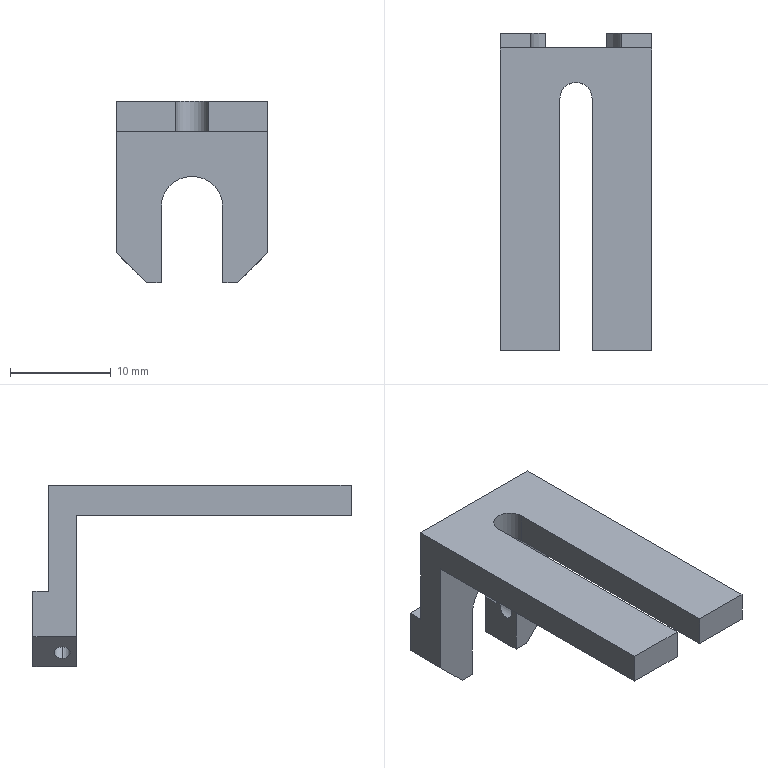Part | SolidWorks | features ICE 6, Extrusion 1, HoleWzd 1, MirrorPattern 1 | 1 solid | 28 faces | box 15 x 31.5 x 18 mm | volume 1594 mm3 | plane 20 | cylinder 8 | commonest cylinder face diameters 1.6 x4 9 x2 3.2 x1 6.1 x1
STEP:
#1=CARTESIAN_POINT('',(-3.05,1.4,-4.353));
#2=VERTEX_POINT('',#1);
#3=CARTESIAN_POINT('',(-3.05,1.4,-2.09));
#4=VERTEX_POINT('',#3);
#5=CARTESIAN_POINT('',(-3.05,1.4,-4.353));
#6=CARTESIAN_POINT('',(-3.05,-0.2,-4.353));
#7=CARTESIAN_POINT('',(-3.05,-0.2,-2.09));
#8=CARTESIAN_POINT('',(-3.05,1.4,-2.09));
#9=(BOUNDED_CURVE()B_SPLINE_CURVE(3,(#5,#6,#7,#8),.UNSPECIFIED.,.F.,.T.)B_SPLINE_CURVE_WITH_KNOTS((4,4),(0.,3.142),.UNSPECIFIED.)CURVE()GEOMETRIC_REPRESENTATION_ITEM()RATIONAL_B_SPLINE_CURVE((1.,0.3333,0.3333,1.))REPRESENTATION_ITEM(''));
#10=EDGE_CURVE('',#2,#4,#9,.T.);
#11=ORIENTED_EDGE('',*,*,#10,.F.);
#12=CARTESIAN_POINT('',(-5.349,1.4,-6.651));
#13=VERTEX_POINT('',#12);
#14=CARTESIAN_POINT('',(-5.349,1.4,-6.651));
#15=DIRECTION('',(-0.7071,0.,-0.7071));
#16=VECTOR('',#15,1000.);
#17=LINE('',#14,#16);
#18=EDGE_CURVE('',#2,#13,#17,.T.);
#19=ORIENTED_EDGE('',*,*,#18,.T.);
#20=CARTESIAN_POINT('',(-6.48,1.4,-5.52));
#21=VERTEX_POINT('',#20);
#22=CARTESIAN_POINT('',(-5.914,1.4,-6.086));
#23=DIRECTION('',(-0.7071,0.,-0.7071));
#24=DIRECTION('',(-0.7071,0.,0.7071));
#25=AXIS2_PLACEMENT_3D('',#22,#23,#24);
#26=CIRCLE('',#25,0.8);
#27=EDGE_CURVE('',#13,#21,#26,.T.);
#28=ORIENTED_EDGE('',*,*,#27,.T.);
#29=CARTESIAN_POINT('',(-6.48,1.4,-5.52));
#30=DIRECTION('',(-0.7071,0.,-0.7071));
#31=VECTOR('',#30,1000.);
#32=LINE('',#29,#31);
#33=EDGE_CURVE('',#4,#21,#32,.T.);
#34=ORIENTED_EDGE('',*,*,#33,.F.);
#35=EDGE_LOOP('',(#11,#19,#28,#34));
#36=FACE_OUTER_BOUND('',#35,.T.);
#37=CARTESIAN_POINT('',(-5.914,1.4,-6.086));
#38=DIRECTION('',(-0.7071,0.,-0.7071));
#39=DIRECTION('',(-0.7071,0.,0.7071));
#40=AXIS2_PLACEMENT_3D('',#37,#38,#39);
#41=CYLINDRICAL_SURFACE('',#40,0.8);
#42=ADVANCED_FACE('',(#36),#41,.F.);
#43=CARTESIAN_POINT('',(3.05,1.4,-2.09));
#44=VERTEX_POINT('',#43);
#45=CARTESIAN_POINT('',(3.05,1.4,-4.353));
#46=VERTEX_POINT('',#45);
#47=CARTESIAN_POINT('',(3.05,1.4,-2.09));
#48=CARTESIAN_POINT('',(3.05,-0.2,-2.09));
#49=CARTESIAN_POINT('',(3.05,-0.2,-4.353));
#50=CARTESIAN_POINT('',(3.05,1.4,-4.353));
#51=(BOUNDED_CURVE()B_SPLINE_CURVE(3,(#47,#48,#49,#50),.UNSPECIFIED.,.F.,.T.)B_SPLINE_CURVE_WITH_KNOTS((4,4),(3.142,6.283),.UNSPECIFIED.)CURVE()GEOMETRIC_REPRESENTATION_ITEM()RATIONAL_B_SPLINE_CURVE((1.,0.3333,0.3333,1.))REPRESENTATION_ITEM(''));
#52=EDGE_CURVE('',#44,#46,#51,.T.);
#53=ORIENTED_EDGE('',*,*,#52,.F.);
#54=CARTESIAN_POINT('',(6.48,1.4,-5.52));
#55=VERTEX_POINT('',#54);
#56=CARTESIAN_POINT('',(6.48,1.4,-5.52));
#57=DIRECTION('',(0.7071,0.,-0.7071));
#58=VECTOR('',#57,1000.);
#59=LINE('',#56,#58);
#60=EDGE_CURVE('',#44,#55,#59,.T.);
#61=ORIENTED_EDGE('',*,*,#60,.T.);
#62=CARTESIAN_POINT('',(5.349,1.4,-6.651));
#63=VERTEX_POINT('',#62);
#64=CARTESIAN_POINT('',(5.914,1.4,-6.086));
#65=DIRECTION('',(0.7071,0.,-0.7071));
#66=DIRECTION('',(-0.7071,0.,-0.7071));
#67=AXIS2_PLACEMENT_3D('',#64,#65,#66);
#68=CIRCLE('',#67,0.8);
#69=EDGE_CURVE('',#55,#63,#68,.T.);
#70=ORIENTED_EDGE('',*,*,#69,.T.);
#71=CARTESIAN_POINT('',(5.349,1.4,-6.651));
#72=DIRECTION('',(0.7071,0.,-0.7071));
#73=VECTOR('',#72,1000.);
#74=LINE('',#71,#73);
#75=EDGE_CURVE('',#46,#63,#74,.T.);
#76=ORIENTED_EDGE('',*,*,#75,.F.);
#77=EDGE_LOOP('',(#53,#61,#70,#76));
#78=FACE_OUTER_BOUND('',#77,.T.);
#79=CARTESIAN_POINT('',(5.914,1.4,-6.086));
#80=DIRECTION('',(0.7071,0.,-0.7071));
#81=DIRECTION('',(-0.7071,0.,-0.7071));
#82=AXIS2_PLACEMENT_3D('',#79,#80,#81);
#83=CYLINDRICAL_SURFACE('',#82,0.8);
#84=ADVANCED_FACE('',(#78),#83,.F.);
#85=CARTESIAN_POINT('',(1.6,-27.2,10.5));
#86=VERTEX_POINT('',#85);
#87=CARTESIAN_POINT('',(7.5,-27.2,10.5));
#88=VERTEX_POINT('',#87);
#89=CARTESIAN_POINT('',(-7.5,-27.2,10.5));
#90=DIRECTION('',(1.,0.,0.));
#91=VECTOR('',#90,1000.);
#92=LINE('',#89,#91);
#93=EDGE_CURVE('',#86,#88,#92,.T.);
#94=ORIENTED_EDGE('',*,*,#93,.F.);
#95=CARTESIAN_POINT('',(1.6,-27.2,7.5));
#96=VERTEX_POINT('',#95);
#97=CARTESIAN_POINT('',(1.6,-27.2,240.5));
#98=DIRECTION('',(0.,0.,-1.));
#99=VECTOR('',#98,1000.);
#100=LINE('',#97,#99);
#101=EDGE_CURVE('',#86,#96,#100,.T.);
#102=ORIENTED_EDGE('',*,*,#101,.T.);
#103=CARTESIAN_POINT('',(7.5,-27.2,7.5));
#104=VERTEX_POINT('',#103);
#105=CARTESIAN_POINT('',(-7.5,-27.2,7.5));
#106=DIRECTION('',(1.,0.,0.));
#107=VECTOR('',#106,1000.);
#108=LINE('',#105,#107);
#109=EDGE_CURVE('',#96,#104,#108,.T.);
#110=ORIENTED_EDGE('',*,*,#109,.T.);
#111=CARTESIAN_POINT('',(7.5,-27.2,10.5));
#112=DIRECTION('',(0.,0.,-1.));
#113=VECTOR('',#112,1000.);
#114=LINE('',#111,#113);
#115=EDGE_CURVE('',#88,#104,#114,.T.);
#116=ORIENTED_EDGE('',*,*,#115,.F.);
#117=EDGE_LOOP('',(#94,#102,#110,#116));
#118=FACE_OUTER_BOUND('',#117,.T.);
#119=CARTESIAN_POINT('',(-7.5,-27.2,10.5));
#120=DIRECTION('',(0.,1.,0.));
#121=DIRECTION('',(0.,0.,1.));
#122=AXIS2_PLACEMENT_3D('',#119,#120,#121);
#123=PLANE('',#122);
#124=ADVANCED_FACE('',(#118),#123,.F.);
#125=CARTESIAN_POINT('',(4.5,2.8,0.));
#126=VERTEX_POINT('',#125);
#127=CARTESIAN_POINT('',(7.5,2.8,0.));
#128=VERTEX_POINT('',#127);
#129=CARTESIAN_POINT('',(0.,2.8,0.));
#130=DIRECTION('',(1.,0.,0.));
#131=VECTOR('',#130,1000.);
#132=LINE('',#129,#131);
#133=EDGE_CURVE('',#126,#128,#132,.T.);
#134=ORIENTED_EDGE('',*,*,#133,.F.);
#135=CARTESIAN_POINT('',(3.05,2.8,-3.309));
#136=VERTEX_POINT('',#135);
#137=CARTESIAN_POINT('',(0.,2.8,0.));
#138=DIRECTION('',(0.,1.,0.));
#139=DIRECTION('',(0.,0.,1.));
#140=AXIS2_PLACEMENT_3D('',#137,#138,#139);
#141=CIRCLE('',#140,4.5);
#142=EDGE_CURVE('',#126,#136,#141,.T.);
#143=ORIENTED_EDGE('',*,*,#142,.T.);
#144=CARTESIAN_POINT('',(3.05,2.8,0.));
#145=VERTEX_POINT('',#144);
#146=CARTESIAN_POINT('',(3.05,2.8,-7.5));
#147=DIRECTION('',(0.,0.,1.));
#148=VECTOR('',#147,1000.);
#149=LINE('',#146,#148);
#150=EDGE_CURVE('',#136,#145,#149,.T.);
#151=ORIENTED_EDGE('',*,*,#150,.T.);
#152=CARTESIAN_POINT('',(-3.05,2.8,0.));
#153=VERTEX_POINT('',#152);
#154=CARTESIAN_POINT('',(0.,2.8,0.));
#155=DIRECTION('',(0.,-1.,0.));
#156=DIRECTION('',(0.,0.,1.));
#157=AXIS2_PLACEMENT_3D('',#154,#155,#156);
#158=CIRCLE('',#157,3.05);
#159=EDGE_CURVE('',#145,#153,#158,.T.);
#160=ORIENTED_EDGE('',*,*,#159,.T.);
#161=CARTESIAN_POINT('',(-3.05,2.8,-3.309));
#162=VERTEX_POINT('',#161);
#163=CARTESIAN_POINT('',(-3.05,2.8,0.));
#164=DIRECTION('',(0.,0.,-1.));
#165=VECTOR('',#164,1000.);
#166=LINE('',#163,#165);
#167=EDGE_CURVE('',#153,#162,#166,.T.);
#168=ORIENTED_EDGE('',*,*,#167,.T.);
#169=CARTESIAN_POINT('',(-4.5,2.8,0.));
#170=VERTEX_POINT('',#169);
#171=CARTESIAN_POINT('',(0.,2.8,0.));
#172=DIRECTION('',(0.,1.,0.));
#173=DIRECTION('',(0.,0.,1.));
#174=AXIS2_PLACEMENT_3D('',#171,#172,#173);
#175=CIRCLE('',#174,4.5);
#176=EDGE_CURVE('',#162,#170,#175,.T.);
#177=ORIENTED_EDGE('',*,*,#176,.T.);
#178=CARTESIAN_POINT('',(-7.5,2.8,0.));
#179=VERTEX_POINT('',#178);
#180=CARTESIAN_POINT('',(0.,2.8,0.));
#181=DIRECTION('',(-1.,0.,0.));
#182=VECTOR('',#181,1000.);
#183=LINE('',#180,#182);
#184=EDGE_CURVE('',#170,#179,#183,.T.);
#185=ORIENTED_EDGE('',*,*,#184,.T.);
#186=CARTESIAN_POINT('',(-7.5,2.8,10.5));
#187=VERTEX_POINT('',#186);
#188=CARTESIAN_POINT('',(-7.5,2.8,7.5));
#189=DIRECTION('',(0.,0.,1.));
#190=VECTOR('',#189,1000.);
#191=LINE('',#188,#190);
#192=EDGE_CURVE('',#179,#187,#191,.T.);
#193=ORIENTED_EDGE('',*,*,#192,.T.);
#194=CARTESIAN_POINT('',(7.5,2.8,10.5));
#195=VERTEX_POINT('',#194);
#196=CARTESIAN_POINT('',(-7.5,2.8,10.5));
#197=DIRECTION('',(-1.,0.,0.));
#198=VECTOR('',#197,1000.);
#199=LINE('',#196,#198);
#200=EDGE_CURVE('',#195,#187,#199,.T.);
#201=ORIENTED_EDGE('',*,*,#200,.F.);
#202=CARTESIAN_POINT('',(7.5,2.8,7.5));
#203=DIRECTION('',(0.,0.,-1.));
#204=VECTOR('',#203,1000.);
#205=LINE('',#202,#204);
#206=EDGE_CURVE('',#195,#128,#205,.T.);
#207=ORIENTED_EDGE('',*,*,#206,.T.);
#208=EDGE_LOOP('',(#134,#143,#151,#160,#168,#177,#185,#193,#201,#207));
#209=FACE_OUTER_BOUND('',#208,.T.);
#210=CARTESIAN_POINT('',(0.,2.8,0.));
#211=DIRECTION('',(0.,1.,0.));
#212=DIRECTION('',(0.,0.,1.));
#213=AXIS2_PLACEMENT_3D('',#210,#211,#212);
#214=PLANE('',#213);
#215=ADVANCED_FACE('',(#209),#214,.T.);
#216=CARTESIAN_POINT('',(3.05,1.4,-4.353));
#217=CARTESIAN_POINT('',(3.05,3.,-4.353));
#218=CARTESIAN_POINT('',(3.05,3.,-2.09));
#219=CARTESIAN_POINT('',(3.05,1.4,-2.09));
#220=(BOUNDED_CURVE()B_SPLINE_CURVE(3,(#216,#217,#218,#219),.UNSPECIFIED.,.F.,.T.)B_SPLINE_CURVE_WITH_KNOTS((4,4),(0.,3.142),.UNSPECIFIED.)CURVE()GEOMETRIC_REPRESENTATION_ITEM()RATIONAL_B_SPLINE_CURVE((1.,0.3333,0.3333,1.))REPRESENTATION_ITEM(''));
#221=EDGE_CURVE('',#46,#44,#220,.T.);
#222=ORIENTED_EDGE('',*,*,#221,.T.);
#223=ORIENTED_EDGE('',*,*,#52,.T.);
#224=EDGE_LOOP('',(#222,#223));
#225=FACE_BOUND('',#224,.T.);
#226=CARTESIAN_POINT('',(3.05,4.3,-3.309));
#227=VERTEX_POINT('',#226);
#228=CARTESIAN_POINT('',(3.05,12.8,-3.309));
#229=DIRECTION('',(0.,-1.,0.));
#230=VECTOR('',#229,1000.);
#231=LINE('',#228,#230);
#232=EDGE_CURVE('',#227,#136,#231,.T.);
#233=ORIENTED_EDGE('',*,*,#232,.F.);
#234=CARTESIAN_POINT('',(3.05,4.3,-7.5));
#235=VERTEX_POINT('',#234);
#236=CARTESIAN_POINT('',(3.05,4.3,-7.5));
#237=DIRECTION('',(0.,0.,1.));
#238=VECTOR('',#237,1000.);
#239=LINE('',#236,#238);
#240=EDGE_CURVE('',#235,#227,#239,.T.);
#241=ORIENTED_EDGE('',*,*,#240,.F.);
#242=CARTESIAN_POINT('',(3.05,0.,-7.5));
#243=VERTEX_POINT('',#242);
#244=CARTESIAN_POINT('',(3.05,2.8,-7.5));
#245=DIRECTION('',(0.,-1.,0.));
#246=VECTOR('',#245,1000.);
#247=LINE('',#244,#246);
#248=EDGE_CURVE('',#235,#243,#247,.T.);
#249=ORIENTED_EDGE('',*,*,#248,.T.);
#250=CARTESIAN_POINT('',(3.05,0.,0.));
#251=VERTEX_POINT('',#250);
#252=CARTESIAN_POINT('',(3.05,0.,-7.5));
#253=DIRECTION('',(0.,0.,1.));
#254=VECTOR('',#253,1000.);
#255=LINE('',#252,#254);
#256=EDGE_CURVE('',#243,#251,#255,.T.);
#257=ORIENTED_EDGE('',*,*,#256,.T.);
#258=CARTESIAN_POINT('',(3.05,2.8,0.));
#259=DIRECTION('',(0.,-1.,0.));
#260=VECTOR('',#259,1000.);
#261=LINE('',#258,#260);
#262=EDGE_CURVE('',#145,#251,#261,.T.);
#263=ORIENTED_EDGE('',*,*,#262,.F.);
#264=ORIENTED_EDGE('',*,*,#150,.F.);
#265=EDGE_LOOP('',(#233,#241,#249,#257,#263,#264));
#266=FACE_OUTER_BOUND('',#265,.T.);
#267=CARTESIAN_POINT('',(3.05,2.8,-7.5));
#268=DIRECTION('',(1.,0.,0.));
#269=DIRECTION('',(0.,0.,-1.));
#270=AXIS2_PLACEMENT_3D('',#267,#268,#269);
#271=PLANE('',#270);
#272=ADVANCED_FACE('',(#225,#266),#271,.F.);
#273=CARTESIAN_POINT('',(-3.05,1.4,-2.09));
#274=CARTESIAN_POINT('',(-3.05,3.,-2.09));
#275=CARTESIAN_POINT('',(-3.05,3.,-4.353));
#276=CARTESIAN_POINT('',(-3.05,1.4,-4.353));
#277=(BOUNDED_CURVE()B_SPLINE_CURVE(3,(#273,#274,#275,#276),.UNSPECIFIED.,.F.,.T.)B_SPLINE_CURVE_WITH_KNOTS((4,4),(3.142,6.283),.UNSPECIFIED.)CURVE()GEOMETRIC_REPRESENTATION_ITEM()RATIONAL_B_SPLINE_CURVE((1.,0.3333,0.3333,1.))REPRESENTATION_ITEM(''));
#278=EDGE_CURVE('',#4,#2,#277,.T.);
#279=ORIENTED_EDGE('',*,*,#278,.T.);
#280=ORIENTED_EDGE('',*,*,#10,.T.);
#281=EDGE_LOOP('',(#279,#280));
#282=FACE_BOUND('',#281,.T.);
#283=CARTESIAN_POINT('',(-3.05,4.3,-3.309));
#284=VERTEX_POINT('',#283);
#285=CARTESIAN_POINT('',(-3.05,12.8,-3.309));
#286=DIRECTION('',(0.,1.,0.));
#287=VECTOR('',#286,1000.);
#288=LINE('',#285,#287);
#289=EDGE_CURVE('',#162,#284,#288,.T.);
#290=ORIENTED_EDGE('',*,*,#289,.F.);
#291=ORIENTED_EDGE('',*,*,#167,.F.);
#292=CARTESIAN_POINT('',(-3.05,0.,0.));
#293=VERTEX_POINT('',#292);
#294=CARTESIAN_POINT('',(-3.05,2.8,0.));
#295=DIRECTION('',(0.,-1.,0.));
#296=VECTOR('',#295,1000.);
#297=LINE('',#294,#296);
#298=EDGE_CURVE('',#153,#293,#297,.T.);
#299=ORIENTED_EDGE('',*,*,#298,.T.);
#300=CARTESIAN_POINT('',(-3.05,0.,-7.5));
#301=VERTEX_POINT('',#300);
#302=CARTESIAN_POINT('',(-3.05,0.,0.));
#303=DIRECTION('',(0.,0.,-1.));
#304=VECTOR('',#303,1000.);
#305=LINE('',#302,#304);
#306=EDGE_CURVE('',#293,#301,#305,.T.);
#307=ORIENTED_EDGE('',*,*,#306,.T.);
#308=CARTESIAN_POINT('',(-3.05,4.3,-7.5));
#309=VERTEX_POINT('',#308);
#310=CARTESIAN_POINT('',(-3.05,2.8,-7.5));
#311=DIRECTION('',(0.,-1.,0.));
#312=VECTOR('',#311,1000.);
#313=LINE('',#310,#312);
#314=EDGE_CURVE('',#309,#301,#313,.T.);
#315=ORIENTED_EDGE('',*,*,#314,.F.);
#316=CARTESIAN_POINT('',(-3.05,4.3,-3.2));
#317=DIRECTION('',(0.,0.,-1.));
#318=VECTOR('',#317,1000.);
#319=LINE('',#316,#318);
#320=EDGE_CURVE('',#284,#309,#319,.T.);
#321=ORIENTED_EDGE('',*,*,#320,.F.);
#322=EDGE_LOOP('',(#290,#291,#299,#307,#315,#321));
#323=FACE_OUTER_BOUND('',#322,.T.);
#324=CARTESIAN_POINT('',(-3.05,2.8,0.));
#325=DIRECTION('',(-1.,0.,0.));
#326=DIRECTION('',(0.,0.,1.));
#327=AXIS2_PLACEMENT_3D('',#324,#325,#326);
#328=PLANE('',#327);
#329=ADVANCED_FACE('',(#282,#323),#328,.F.);
#330=CARTESIAN_POINT('',(4.5,4.3,-7.5));
#331=VERTEX_POINT('',#330);
#332=CARTESIAN_POINT('',(7.5,4.3,-7.5));
#333=DIRECTION('',(-1.,0.,0.));
#334=VECTOR('',#333,1000.);
#335=LINE('',#332,#334);
#336=EDGE_CURVE('',#331,#235,#335,.T.);
#337=ORIENTED_EDGE('',*,*,#336,.F.);
#338=CARTESIAN_POINT('',(4.5,0.,-7.5));
#339=VERTEX_POINT('',#338);
#340=CARTESIAN_POINT('',(4.5,0.,-7.5));
#341=DIRECTION('',(0.,1.,0.));
#342=VECTOR('',#341,1000.);
#343=LINE('',#340,#342);
#344=EDGE_CURVE('',#339,#331,#343,.T.);
#345=ORIENTED_EDGE('',*,*,#344,.F.);
#346=CARTESIAN_POINT('',(3.05,0.,-7.5));
#347=DIRECTION('',(-1.,0.,0.));
#348=VECTOR('',#347,1000.);
#349=LINE('',#346,#348);
#350=EDGE_CURVE('',#339,#243,#349,.T.);
#351=ORIENTED_EDGE('',*,*,#350,.T.);
#352=ORIENTED_EDGE('',*,*,#248,.F.);
#353=EDGE_LOOP('',(#337,#345,#351,#352));
#354=FACE_OUTER_BOUND('',#353,.T.);
#355=CARTESIAN_POINT('',(3.05,2.8,-7.5));
#356=DIRECTION('',(0.,0.,1.));
#357=DIRECTION('',(1.,0.,0.));
#358=AXIS2_PLACEMENT_3D('',#355,#356,#357);
#359=PLANE('',#358);
#360=ADVANCED_FACE('',(#354),#359,.F.);
#361=CARTESIAN_POINT('',(0.,0.,0.));
#362=DIRECTION('',(0.,-1.,0.));
#363=DIRECTION('',(0.,0.,1.));
#364=AXIS2_PLACEMENT_3D('',#361,#362,#363);
#365=CIRCLE('',#364,3.05);
#366=EDGE_CURVE('',#251,#293,#365,.T.);
#367=ORIENTED_EDGE('',*,*,#366,.T.);
#368=ORIENTED_EDGE('',*,*,#298,.F.);
#369=ORIENTED_EDGE('',*,*,#159,.F.);
#370=ORIENTED_EDGE('',*,*,#262,.T.);
#371=EDGE_LOOP('',(#367,#368,#369,#370));
#372=FACE_OUTER_BOUND('',#371,.T.);
#373=CARTESIAN_POINT('',(0.,2.8,0.));
#374=DIRECTION('',(0.,-1.,0.));
#375=DIRECTION('',(0.,0.,-1.));
#376=AXIS2_PLACEMENT_3D('',#373,#374,#375);
#377=CYLINDRICAL_SURFACE('',#376,3.05);
#378=ADVANCED_FACE('',(#372),#377,.F.);
#379=CARTESIAN_POINT('',(-4.5,0.,-7.5));
#380=VERTEX_POINT('',#379);
#381=CARTESIAN_POINT('',(-7.5,0.,-7.5));
#382=DIRECTION('',(-1.,0.,0.));
#383=VECTOR('',#382,1000.);
#384=LINE('',#381,#383);
#385=EDGE_CURVE('',#301,#380,#384,.T.);
#386=ORIENTED_EDGE('',*,*,#385,.T.);
#387=CARTESIAN_POINT('',(-4.5,4.3,-7.5));
#388=VERTEX_POINT('',#387);
#389=CARTESIAN_POINT('',(-4.5,0.,-7.5));
#390=DIRECTION('',(0.,1.,0.));
#391=VECTOR('',#390,1000.);
#392=LINE('',#389,#391);
#393=EDGE_CURVE('',#380,#388,#392,.T.);
#394=ORIENTED_EDGE('',*,*,#393,.T.);
#395=CARTESIAN_POINT('',(-3.05,4.3,-7.5));
#396=DIRECTION('',(-1.,0.,0.));
#397=VECTOR('',#396,1000.);
#398=LINE('',#395,#397);
#399=EDGE_CURVE('',#309,#388,#398,.T.);
#400=ORIENTED_EDGE('',*,*,#399,.F.);
#401=ORIENTED_EDGE('',*,*,#314,.T.);
#402=EDGE_LOOP('',(#386,#394,#400,#401));
#403=FACE_OUTER_BOUND('',#402,.T.);
#404=CARTESIAN_POINT('',(-7.5,2.8,-7.5));
#405=DIRECTION('',(0.,0.,1.));
#406=DIRECTION('',(1.,0.,0.));
#407=AXIS2_PLACEMENT_3D('',#404,#405,#406);
#408=PLANE('',#407);
#409=ADVANCED_FACE('',(#403),#408,.F.);
#410=CARTESIAN_POINT('',(-7.5,4.3,-4.5));
#411=VERTEX_POINT('',#410);
#412=CARTESIAN_POINT('',(-7.5,4.3,0.));
#413=VERTEX_POINT('',#412);
#414=CARTESIAN_POINT('',(-7.5,4.3,-7.5));
#415=DIRECTION('',(0.,0.,1.));
#416=VECTOR('',#415,1000.);
#417=LINE('',#414,#416);
#418=EDGE_CURVE('',#411,#413,#417,.T.);
#419=ORIENTED_EDGE('',*,*,#418,.F.);
#420=CARTESIAN_POINT('',(-7.5,0.,-4.5));
#421=VERTEX_POINT('',#420);
#422=CARTESIAN_POINT('',(-7.5,0.,-4.5));
#423=DIRECTION('',(0.,1.,0.));
#424=VECTOR('',#423,1000.);
#425=LINE('',#422,#424);
#426=EDGE_CURVE('',#421,#411,#425,.T.);
#427=ORIENTED_EDGE('',*,*,#426,.F.);
#428=CARTESIAN_POINT('',(-7.5,0.,7.5));
#429=VERTEX_POINT('',#428);
#430=CARTESIAN_POINT('',(-7.5,0.,7.5));
#431=DIRECTION('',(0.,0.,1.));
#432=VECTOR('',#431,1000.);
#433=LINE('',#430,#432);
#434=EDGE_CURVE('',#421,#429,#433,.T.);
#435=ORIENTED_EDGE('',*,*,#434,.T.);
#436=CARTESIAN_POINT('',(-7.5,-27.2,7.5));
#437=VERTEX_POINT('',#436);
#438=CARTESIAN_POINT('',(-7.5,2.8,7.5));
#439=DIRECTION('',(0.,-1.,0.));
#440=VECTOR('',#439,1000.);
#441=LINE('',#438,#440);
#442=EDGE_CURVE('',#429,#437,#441,.T.);
#443=ORIENTED_EDGE('',*,*,#442,.T.);
#444=CARTESIAN_POINT('',(-7.5,-27.2,10.5));
#445=VERTEX_POINT('',#444);
#446=CARTESIAN_POINT('',(-7.5,-27.2,10.5));
#447=DIRECTION('',(0.,0.,-1.));
#448=VECTOR('',#447,1000.);
#449=LINE('',#446,#448);
#450=EDGE_CURVE('',#445,#437,#449,.T.);
#451=ORIENTED_EDGE('',*,*,#450,.F.);
#452=CARTESIAN_POINT('',(-7.5,2.8,10.5));
#453=DIRECTION('',(0.,-1.,0.));
#454=VECTOR('',#453,1000.);
#455=LINE('',#452,#454);
#456=EDGE_CURVE('',#187,#445,#455,.T.);
#457=ORIENTED_EDGE('',*,*,#456,.F.);
#458=ORIENTED_EDGE('',*,*,#192,.F.);
#459=CARTESIAN_POINT('',(-7.5,9.689,0.));
#460=DIRECTION('',(0.,-1.,0.));
#461=VECTOR('',#460,1000.);
#462=LINE('',#459,#461);
#463=EDGE_CURVE('',#413,#179,#462,.T.);
#464=ORIENTED_EDGE('',*,*,#463,.F.);
#465=EDGE_LOOP('',(#419,#427,#435,#443,#451,#457,#458,#464));
#466=FACE_OUTER_BOUND('',#465,.T.);
#467=CARTESIAN_POINT('',(-7.5,2.8,7.5));
#468=DIRECTION('',(1.,0.,0.));
#469=DIRECTION('',(0.,0.,-1.));
#470=AXIS2_PLACEMENT_3D('',#467,#468,#469);
#471=PLANE('',#470);
#472=ADVANCED_FACE('',(#466),#471,.F.);
#473=CARTESIAN_POINT('',(7.5,0.,7.5));
#474=VERTEX_POINT('',#473);
#475=CARTESIAN_POINT('',(7.5,0.,-4.5));
#476=VERTEX_POINT('',#475);
#477=CARTESIAN_POINT('',(7.5,0.,7.5));
#478=DIRECTION('',(0.,0.,-1.));
#479=VECTOR('',#478,1000.);
#480=LINE('',#477,#479);
#481=EDGE_CURVE('',#474,#476,#480,.T.);
#482=ORIENTED_EDGE('',*,*,#481,.T.);
#483=CARTESIAN_POINT('',(7.5,4.3,-4.5));
#484=VERTEX_POINT('',#483);
#485=CARTESIAN_POINT('',(7.5,0.,-4.5));
#486=DIRECTION('',(0.,1.,0.));
#487=VECTOR('',#486,1000.);
#488=LINE('',#485,#487);
#489=EDGE_CURVE('',#476,#484,#488,.T.);
#490=ORIENTED_EDGE('',*,*,#489,.T.);
#491=CARTESIAN_POINT('',(7.5,4.3,0.));
#492=VERTEX_POINT('',#491);
#493=CARTESIAN_POINT('',(7.5,4.3,-3.2));
#494=DIRECTION('',(0.,0.,-1.));
#495=VECTOR('',#494,1000.);
#496=LINE('',#493,#495);
#497=EDGE_CURVE('',#492,#484,#496,.T.);
#498=ORIENTED_EDGE('',*,*,#497,.F.);
#499=CARTESIAN_POINT('',(7.5,9.689,0.));
#500=DIRECTION('',(0.,-1.,0.));
#501=VECTOR('',#500,1000.);
#502=LINE('',#499,#501);
#503=EDGE_CURVE('',#492,#128,#502,.T.);
#504=ORIENTED_EDGE('',*,*,#503,.T.);
#505=ORIENTED_EDGE('',*,*,#206,.F.);
#506=CARTESIAN_POINT('',(7.5,2.8,10.5));
#507=DIRECTION('',(0.,1.,0.));
#508=VECTOR('',#507,1000.);
#509=LINE('',#506,#508);
#510=EDGE_CURVE('',#88,#195,#509,.T.);
#511=ORIENTED_EDGE('',*,*,#510,.F.);
#512=ORIENTED_EDGE('',*,*,#115,.T.);
#513=CARTESIAN_POINT('',(7.5,2.8,7.5));
#514=DIRECTION('',(0.,1.,0.));
#515=VECTOR('',#514,1000.);
#516=LINE('',#513,#515);
#517=EDGE_CURVE('',#104,#474,#516,.T.);
#518=ORIENTED_EDGE('',*,*,#517,.T.);
#519=EDGE_LOOP('',(#482,#490,#498,#504,#505,#511,#512,#518));
#520=FACE_OUTER_BOUND('',#519,.T.);
#521=CARTESIAN_POINT('',(7.5,2.8,7.5));
#522=DIRECTION('',(-1.,0.,0.));
#523=DIRECTION('',(0.,0.,1.));
#524=AXIS2_PLACEMENT_3D('',#521,#522,#523);
#525=PLANE('',#524);
#526=ADVANCED_FACE('',(#520),#525,.F.);
#527=ORIENTED_EDGE('',*,*,#350,.F.);
#528=CARTESIAN_POINT('',(4.5,0.,-7.5));
#529=DIRECTION('',(0.7071,0.,0.7071));
#530=VECTOR('',#529,1000.);
#531=LINE('',#528,#530);
#532=EDGE_CURVE('',#339,#476,#531,.T.);
#533=ORIENTED_EDGE('',*,*,#532,.T.);
#534=ORIENTED_EDGE('',*,*,#481,.F.);
#535=CARTESIAN_POINT('',(-7.5,0.,7.5));
#536=DIRECTION('',(1.,0.,0.));
#537=VECTOR('',#536,1000.);
#538=LINE('',#535,#537);
#539=EDGE_CURVE('',#429,#474,#538,.T.);
#540=ORIENTED_EDGE('',*,*,#539,.F.);
#541=ORIENTED_EDGE('',*,*,#434,.F.);
#542=CARTESIAN_POINT('',(-4.5,0.,-7.5));
#543=DIRECTION('',(0.7071,0.,-0.7071));
#544=VECTOR('',#543,1000.);
#545=LINE('',#542,#544);
#546=EDGE_CURVE('',#421,#380,#545,.T.);
#547=ORIENTED_EDGE('',*,*,#546,.T.);
#548=ORIENTED_EDGE('',*,*,#385,.F.);
#549=ORIENTED_EDGE('',*,*,#306,.F.);
#550=ORIENTED_EDGE('',*,*,#366,.F.);
#551=ORIENTED_EDGE('',*,*,#256,.F.);
#552=EDGE_LOOP('',(#527,#533,#534,#540,#541,#547,#548,#549,#550,#551));
#553=FACE_OUTER_BOUND('',#552,.T.);
#554=CARTESIAN_POINT('',(0.,0.,0.));
#555=DIRECTION('',(0.,1.,0.));
#556=DIRECTION('',(0.,0.,1.));
#557=AXIS2_PLACEMENT_3D('',#554,#555,#556);
#558=PLANE('',#557);
#559=ADVANCED_FACE('',(#553),#558,.F.);
#560=CARTESIAN_POINT('',(-4.5,4.3,-7.5));
#561=DIRECTION('',(0.7071,0.,-0.7071));
#562=VECTOR('',#561,1000.);
#563=LINE('',#560,#562);
#564=EDGE_CURVE('',#411,#388,#563,.T.);
#565=ORIENTED_EDGE('',*,*,#564,.F.);
#566=ORIENTED_EDGE('',*,*,#418,.T.);
#567=CARTESIAN_POINT('',(-4.5,4.3,0.));
#568=VERTEX_POINT('',#567);
#569=CARTESIAN_POINT('',(0.,4.3,0.));
#570=DIRECTION('',(-1.,0.,0.));
#571=VECTOR('',#570,1000.);
#572=LINE('',#569,#571);
#573=EDGE_CURVE('',#568,#413,#572,.T.);
#574=ORIENTED_EDGE('',*,*,#573,.F.);
#575=CARTESIAN_POINT('',(0.,4.3,0.));
#576=DIRECTION('',(0.,-1.,0.));
#577=DIRECTION('',(0.,0.,1.));
#578=AXIS2_PLACEMENT_3D('',#575,#576,#577);
#579=CIRCLE('',#578,4.5);
#580=EDGE_CURVE('',#568,#284,#579,.T.);
#581=ORIENTED_EDGE('',*,*,#580,.T.);
#582=ORIENTED_EDGE('',*,*,#320,.T.);
#583=ORIENTED_EDGE('',*,*,#399,.T.);
#584=EDGE_LOOP('',(#565,#566,#574,#581,#582,#583));
#585=FACE_OUTER_BOUND('',#584,.T.);
#586=CARTESIAN_POINT('',(0.,4.3,0.));
#587=DIRECTION('',(0.,1.,0.));
#588=DIRECTION('',(0.,0.,1.));
#589=AXIS2_PLACEMENT_3D('',#586,#587,#588);
#590=PLANE('',#589);
#591=ADVANCED_FACE('',(#585),#590,.T.);
#592=CARTESIAN_POINT('',(4.5,4.3,-7.5));
#593=DIRECTION('',(0.7071,0.,0.7071));
#594=VECTOR('',#593,1000.);
#595=LINE('',#592,#594);
#596=EDGE_CURVE('',#331,#484,#595,.T.);
#597=ORIENTED_EDGE('',*,*,#596,.F.);
#598=ORIENTED_EDGE('',*,*,#336,.T.);
#599=ORIENTED_EDGE('',*,*,#240,.T.);
#600=CARTESIAN_POINT('',(4.5,4.3,0.));
#601=VERTEX_POINT('',#600);
#602=CARTESIAN_POINT('',(0.,4.3,0.));
#603=DIRECTION('',(0.,-1.,0.));
#604=DIRECTION('',(0.,0.,1.));
#605=AXIS2_PLACEMENT_3D('',#602,#603,#604);
#606=CIRCLE('',#605,4.5);
#607=EDGE_CURVE('',#227,#601,#606,.T.);
#608=ORIENTED_EDGE('',*,*,#607,.T.);
#609=CARTESIAN_POINT('',(0.,4.3,0.));
#610=DIRECTION('',(1.,0.,0.));
#611=VECTOR('',#610,1000.);
#612=LINE('',#609,#611);
#613=EDGE_CURVE('',#601,#492,#612,.T.);
#614=ORIENTED_EDGE('',*,*,#613,.T.);
#615=ORIENTED_EDGE('',*,*,#497,.T.);
#616=EDGE_LOOP('',(#597,#598,#599,#608,#614,#615));
#617=FACE_OUTER_BOUND('',#616,.T.);
#618=CARTESIAN_POINT('',(0.,4.3,0.));
#619=DIRECTION('',(0.,1.,0.));
#620=DIRECTION('',(0.,0.,1.));
#621=AXIS2_PLACEMENT_3D('',#618,#619,#620);
#622=PLANE('',#621);
#623=ADVANCED_FACE('',(#617),#622,.T.);
#624=ORIENTED_EDGE('',*,*,#232,.T.);
#625=ORIENTED_EDGE('',*,*,#142,.F.);
#626=CARTESIAN_POINT('',(4.5,9.689,0.));
#627=DIRECTION('',(0.,-1.,0.));
#628=VECTOR('',#627,1000.);
#629=LINE('',#626,#628);
#630=EDGE_CURVE('',#601,#126,#629,.T.);
#631=ORIENTED_EDGE('',*,*,#630,.F.);
#632=ORIENTED_EDGE('',*,*,#607,.F.);
#633=EDGE_LOOP('',(#624,#625,#631,#632));
#634=FACE_OUTER_BOUND('',#633,.T.);
#635=CARTESIAN_POINT('',(0.,12.8,0.));
#636=DIRECTION('',(0.,-1.,0.));
#637=DIRECTION('',(0.,0.,-1.));
#638=AXIS2_PLACEMENT_3D('',#635,#636,#637);
#639=CYLINDRICAL_SURFACE('',#638,4.5);
#640=ADVANCED_FACE('',(#634),#639,.F.);
#641=ORIENTED_EDGE('',*,*,#289,.T.);
#642=ORIENTED_EDGE('',*,*,#580,.F.);
#643=CARTESIAN_POINT('',(-4.5,9.689,0.));
#644=DIRECTION('',(0.,-1.,0.));
#645=VECTOR('',#644,1000.);
#646=LINE('',#643,#645);
#647=EDGE_CURVE('',#568,#170,#646,.T.);
#648=ORIENTED_EDGE('',*,*,#647,.T.);
#649=ORIENTED_EDGE('',*,*,#176,.F.);
#650=EDGE_LOOP('',(#641,#642,#648,#649));
#651=FACE_OUTER_BOUND('',#650,.T.);
#652=CARTESIAN_POINT('',(0.,12.8,0.));
#653=DIRECTION('',(0.,-1.,0.));
#654=DIRECTION('',(0.,0.,-1.));
#655=AXIS2_PLACEMENT_3D('',#652,#653,#654);
#656=CYLINDRICAL_SURFACE('',#655,4.5);
#657=ADVANCED_FACE('',(#651),#656,.F.);
#658=ORIENTED_EDGE('',*,*,#647,.F.);
#659=ORIENTED_EDGE('',*,*,#573,.T.);
#660=ORIENTED_EDGE('',*,*,#463,.T.);
#661=ORIENTED_EDGE('',*,*,#184,.F.);
#662=EDGE_LOOP('',(#658,#659,#660,#661));
#663=FACE_OUTER_BOUND('',#662,.T.);
#664=CARTESIAN_POINT('',(0.,9.689,0.));
#665=DIRECTION('',(0.,0.,1.));
#666=DIRECTION('',(1.,0.,0.));
#667=AXIS2_PLACEMENT_3D('',#664,#665,#666);
#668=PLANE('',#667);
#669=ADVANCED_FACE('',(#663),#668,.T.);
#670=ORIENTED_EDGE('',*,*,#613,.F.);
#671=ORIENTED_EDGE('',*,*,#630,.T.);
#672=ORIENTED_EDGE('',*,*,#133,.T.);
#673=ORIENTED_EDGE('',*,*,#503,.F.);
#674=EDGE_LOOP('',(#670,#671,#672,#673));
#675=FACE_OUTER_BOUND('',#674,.T.);
#676=CARTESIAN_POINT('',(0.,9.689,0.));
#677=DIRECTION('',(0.,0.,-1.));
#678=DIRECTION('',(-1.,0.,0.));
#679=AXIS2_PLACEMENT_3D('',#676,#677,#678);
#680=PLANE('',#679);
#681=ADVANCED_FACE('',(#675),#680,.F.);
#682=CARTESIAN_POINT('',(5.914,1.4,-6.086));
#683=DIRECTION('',(0.7071,0.,-0.7071));
#684=DIRECTION('',(-0.7071,0.,-0.7071));
#685=AXIS2_PLACEMENT_3D('',#682,#683,#684);
#686=CIRCLE('',#685,0.8);
#687=EDGE_CURVE('',#63,#55,#686,.T.);
#688=ORIENTED_EDGE('',*,*,#687,.F.);
#689=ORIENTED_EDGE('',*,*,#69,.F.);
#690=EDGE_LOOP('',(#688,#689));
#691=FACE_BOUND('',#690,.T.);
#692=ORIENTED_EDGE('',*,*,#596,.T.);
#693=ORIENTED_EDGE('',*,*,#489,.F.);
#694=ORIENTED_EDGE('',*,*,#532,.F.);
#695=ORIENTED_EDGE('',*,*,#344,.T.);
#696=EDGE_LOOP('',(#692,#693,#694,#695));
#697=FACE_OUTER_BOUND('',#696,.T.);
#698=CARTESIAN_POINT('',(4.5,0.,-7.5));
#699=DIRECTION('',(-0.7071,0.,0.7071));
#700=DIRECTION('',(0.7071,0.,0.7071));
#701=AXIS2_PLACEMENT_3D('',#698,#699,#700);
#702=PLANE('',#701);
#703=ADVANCED_FACE('',(#691,#697),#702,.F.);
#704=CARTESIAN_POINT('',(-5.914,1.4,-6.086));
#705=DIRECTION('',(-0.7071,0.,-0.7071));
#706=DIRECTION('',(-0.7071,0.,0.7071));
#707=AXIS2_PLACEMENT_3D('',#704,#705,#706);
#708=CIRCLE('',#707,0.8);
#709=EDGE_CURVE('',#21,#13,#708,.T.);
#710=ORIENTED_EDGE('',*,*,#709,.F.);
#711=ORIENTED_EDGE('',*,*,#27,.F.);
#712=EDGE_LOOP('',(#710,#711));
#713=FACE_BOUND('',#712,.T.);
#714=ORIENTED_EDGE('',*,*,#564,.T.);
#715=ORIENTED_EDGE('',*,*,#393,.F.);
#716=ORIENTED_EDGE('',*,*,#546,.F.);
#717=ORIENTED_EDGE('',*,*,#426,.T.);
#718=EDGE_LOOP('',(#714,#715,#716,#717));
#719=FACE_OUTER_BOUND('',#718,.T.);
#720=CARTESIAN_POINT('',(-4.5,0.,-7.5));
#721=DIRECTION('',(0.7071,0.,0.7071));
#722=DIRECTION('',(0.7071,0.,-0.7071));
#723=AXIS2_PLACEMENT_3D('',#720,#721,#722);
#724=PLANE('',#723);
#725=ADVANCED_FACE('',(#713,#719),#724,.F.);
#726=ORIENTED_EDGE('',*,*,#60,.F.);
#727=ORIENTED_EDGE('',*,*,#221,.F.);
#728=ORIENTED_EDGE('',*,*,#75,.T.);
#729=ORIENTED_EDGE('',*,*,#687,.T.);
#730=EDGE_LOOP('',(#726,#727,#728,#729));
#731=FACE_OUTER_BOUND('',#730,.T.);
#732=CARTESIAN_POINT('',(5.914,1.4,-6.086));
#733=DIRECTION('',(0.7071,0.,-0.7071));
#734=DIRECTION('',(-0.7071,0.,-0.7071));
#735=AXIS2_PLACEMENT_3D('',#732,#733,#734);
#736=CYLINDRICAL_SURFACE('',#735,0.8);
#737=ADVANCED_FACE('',(#731),#736,.F.);
#738=ORIENTED_EDGE('',*,*,#18,.F.);
#739=ORIENTED_EDGE('',*,*,#278,.F.);
#740=ORIENTED_EDGE('',*,*,#33,.T.);
#741=ORIENTED_EDGE('',*,*,#709,.T.);
#742=EDGE_LOOP('',(#738,#739,#740,#741));
#743=FACE_OUTER_BOUND('',#742,.T.);
#744=CARTESIAN_POINT('',(-5.914,1.4,-6.086));
#745=DIRECTION('',(-0.7071,0.,-0.7071));
#746=DIRECTION('',(-0.7071,0.,0.7071));
#747=AXIS2_PLACEMENT_3D('',#744,#745,#746);
#748=CYLINDRICAL_SURFACE('',#747,0.8);
#749=ADVANCED_FACE('',(#743),#748,.F.);
#750=ORIENTED_EDGE('',*,*,#109,.F.);
#751=CARTESIAN_POINT('',(1.6,-2.2,7.5));
#752=VERTEX_POINT('',#751);
#753=CARTESIAN_POINT('',(1.6,-27.2,7.5));
#754=DIRECTION('',(0.,-1.,0.));
#755=VECTOR('',#754,1000.);
#756=LINE('',#753,#755);
#757=EDGE_CURVE('',#752,#96,#756,.T.);
#758=ORIENTED_EDGE('',*,*,#757,.F.);
#759=CARTESIAN_POINT('',(-1.6,-2.2,7.5));
#760=VERTEX_POINT('',#759);
#761=CARTESIAN_POINT('',(0.,-2.2,7.5));
#762=DIRECTION('',(0.,0.,-1.));
#763=DIRECTION('',(-1.,0.,0.));
#764=AXIS2_PLACEMENT_3D('',#761,#762,#763);
#765=CIRCLE('',#764,1.6);
#766=EDGE_CURVE('',#760,#752,#765,.T.);
#767=ORIENTED_EDGE('',*,*,#766,.F.);
#768=CARTESIAN_POINT('',(-1.6,-27.2,7.5));
#769=VERTEX_POINT('',#768);
#770=CARTESIAN_POINT('',(-1.6,-27.2,7.5));
#771=DIRECTION('',(0.,1.,0.));
#772=VECTOR('',#771,1000.);
#773=LINE('',#770,#772);
#774=EDGE_CURVE('',#769,#760,#773,.T.);
#775=ORIENTED_EDGE('',*,*,#774,.F.);
#776=CARTESIAN_POINT('',(-7.5,-27.2,7.5));
#777=DIRECTION('',(1.,0.,0.));
#778=VECTOR('',#777,1000.);
#779=LINE('',#776,#778);
#780=EDGE_CURVE('',#437,#769,#779,.T.);
#781=ORIENTED_EDGE('',*,*,#780,.F.);
#782=ORIENTED_EDGE('',*,*,#442,.F.);
#783=ORIENTED_EDGE('',*,*,#539,.T.);
#784=ORIENTED_EDGE('',*,*,#517,.F.);
#785=EDGE_LOOP('',(#750,#758,#767,#775,#781,#782,#783,#784));
#786=FACE_OUTER_BOUND('',#785,.T.);
#787=CARTESIAN_POINT('',(0.,0.,7.5));
#788=DIRECTION('',(0.,0.,1.));
#789=DIRECTION('',(1.,0.,0.));
#790=AXIS2_PLACEMENT_3D('',#787,#788,#789);
#791=PLANE('',#790);
#792=ADVANCED_FACE('',(#786),#791,.F.);
#793=ORIENTED_EDGE('',*,*,#780,.T.);
#794=CARTESIAN_POINT('',(-1.6,-27.2,10.5));
#795=VERTEX_POINT('',#794);
#796=CARTESIAN_POINT('',(-1.6,-27.2,240.5));
#797=DIRECTION('',(0.,0.,-1.));
#798=VECTOR('',#797,1000.);
#799=LINE('',#796,#798);
#800=EDGE_CURVE('',#795,#769,#799,.T.);
#801=ORIENTED_EDGE('',*,*,#800,.F.);
#802=CARTESIAN_POINT('',(-7.5,-27.2,10.5));
#803=DIRECTION('',(1.,0.,0.));
#804=VECTOR('',#803,1000.);
#805=LINE('',#802,#804);
#806=EDGE_CURVE('',#445,#795,#805,.T.);
#807=ORIENTED_EDGE('',*,*,#806,.F.);
#808=ORIENTED_EDGE('',*,*,#450,.T.);
#809=EDGE_LOOP('',(#793,#801,#807,#808));
#810=FACE_OUTER_BOUND('',#809,.T.);
#811=CARTESIAN_POINT('',(-7.5,-27.2,10.5));
#812=DIRECTION('',(0.,1.,0.));
#813=DIRECTION('',(0.,0.,1.));
#814=AXIS2_PLACEMENT_3D('',#811,#812,#813);
#815=PLANE('',#814);
#816=ADVANCED_FACE('',(#810),#815,.F.);
#817=CARTESIAN_POINT('',(1.6,-2.2,10.5));
#818=VERTEX_POINT('',#817);
#819=CARTESIAN_POINT('',(1.6,0.,10.5));
#820=DIRECTION('',(0.,1.,0.));
#821=VECTOR('',#820,1000.);
#822=LINE('',#819,#821);
#823=EDGE_CURVE('',#86,#818,#822,.T.);
#824=ORIENTED_EDGE('',*,*,#823,.F.);
#825=ORIENTED_EDGE('',*,*,#93,.T.);
#826=ORIENTED_EDGE('',*,*,#510,.T.);
#827=ORIENTED_EDGE('',*,*,#200,.T.);
#828=ORIENTED_EDGE('',*,*,#456,.T.);
#829=ORIENTED_EDGE('',*,*,#806,.T.);
#830=CARTESIAN_POINT('',(-1.6,-2.2,10.5));
#831=VERTEX_POINT('',#830);
#832=CARTESIAN_POINT('',(-1.6,0.,10.5));
#833=DIRECTION('',(0.,-1.,0.));
#834=VECTOR('',#833,1000.);
#835=LINE('',#832,#834);
#836=EDGE_CURVE('',#831,#795,#835,.T.);
#837=ORIENTED_EDGE('',*,*,#836,.F.);
#838=CARTESIAN_POINT('',(0.,-2.2,10.5));
#839=DIRECTION('',(0.,0.,1.));
#840=DIRECTION('',(1.,0.,0.));
#841=AXIS2_PLACEMENT_3D('',#838,#839,#840);
#842=CIRCLE('',#841,1.6);
#843=EDGE_CURVE('',#818,#831,#842,.T.);
#844=ORIENTED_EDGE('',*,*,#843,.F.);
#845=EDGE_LOOP('',(#824,#825,#826,#827,#828,#829,#837,#844));
#846=FACE_OUTER_BOUND('',#845,.T.);
#847=CARTESIAN_POINT('',(0.,0.,10.5));
#848=DIRECTION('',(0.,0.,1.));
#849=DIRECTION('',(1.,0.,0.));
#850=AXIS2_PLACEMENT_3D('',#847,#848,#849);
#851=PLANE('',#850);
#852=ADVANCED_FACE('',(#846),#851,.T.);
#853=ORIENTED_EDGE('',*,*,#823,.T.);
#854=CARTESIAN_POINT('',(1.6,-2.2,240.5));
#855=DIRECTION('',(0.,0.,-1.));
#856=VECTOR('',#855,1000.);
#857=LINE('',#854,#856);
#858=EDGE_CURVE('',#818,#752,#857,.T.);
#859=ORIENTED_EDGE('',*,*,#858,.T.);
#860=ORIENTED_EDGE('',*,*,#757,.T.);
#861=ORIENTED_EDGE('',*,*,#101,.F.);
#862=EDGE_LOOP('',(#853,#859,#860,#861));
#863=FACE_OUTER_BOUND('',#862,.T.);
#864=CARTESIAN_POINT('',(1.6,-27.2,240.5));
#865=DIRECTION('',(1.,0.,0.));
#866=DIRECTION('',(0.,0.,-1.));
#867=AXIS2_PLACEMENT_3D('',#864,#865,#866);
#868=PLANE('',#867);
#869=ADVANCED_FACE('',(#863),#868,.F.);
#870=ORIENTED_EDGE('',*,*,#843,.T.);
#871=CARTESIAN_POINT('',(-1.6,-2.2,240.5));
#872=DIRECTION('',(0.,0.,-1.));
#873=VECTOR('',#872,1000.);
#874=LINE('',#871,#873);
#875=EDGE_CURVE('',#831,#760,#874,.T.);
#876=ORIENTED_EDGE('',*,*,#875,.T.);
#877=ORIENTED_EDGE('',*,*,#766,.T.);
#878=ORIENTED_EDGE('',*,*,#858,.F.);
#879=EDGE_LOOP('',(#870,#876,#877,#878));
#880=FACE_OUTER_BOUND('',#879,.T.);
#881=CARTESIAN_POINT('',(0.,-2.2,240.5));
#882=DIRECTION('',(0.,0.,-1.));
#883=DIRECTION('',(-1.,0.,0.));
#884=AXIS2_PLACEMENT_3D('',#881,#882,#883);
#885=CYLINDRICAL_SURFACE('',#884,1.6);
#886=ADVANCED_FACE('',(#880),#885,.F.);
#887=ORIENTED_EDGE('',*,*,#836,.T.);
#888=ORIENTED_EDGE('',*,*,#800,.T.);
#889=ORIENTED_EDGE('',*,*,#774,.T.);
#890=ORIENTED_EDGE('',*,*,#875,.F.);
#891=EDGE_LOOP('',(#887,#888,#889,#890));
#892=FACE_OUTER_BOUND('',#891,.T.);
#893=CARTESIAN_POINT('',(-1.6,-27.2,240.5));
#894=DIRECTION('',(-1.,0.,0.));
#895=DIRECTION('',(0.,0.,1.));
#896=AXIS2_PLACEMENT_3D('',#893,#894,#895);
#897=PLANE('',#896);
#898=ADVANCED_FACE('',(#892),#897,.F.);
#899=CLOSED_SHELL('',(#42,#84,#124,#215,#272,#329,#360,#378,#409,#472,#526,#559,#591,#623,#640,#657,#669,#681,#703,#725,#737,#749,#792,#816,#852,#869,#886,#898));
#900=MANIFOLD_SOLID_BREP('',#899);
#901=CARTESIAN_POINT('',(0.,0.,0.));
#902=DIRECTION('',(0.,0.,1.));
#903=DIRECTION('',(1.,0.,0.));
#904=AXIS2_PLACEMENT_3D('',#901,#902,#903);
#905=(LENGTH_UNIT()NAMED_UNIT(*)SI_UNIT(.MILLI.,.METRE.));
#906=UNCERTAINTY_MEASURE_WITH_UNIT(LENGTH_MEASURE(0.00001),#905,'','');
#907=(NAMED_UNIT(*)PLANE_ANGLE_UNIT()SI_UNIT($,.RADIAN.));
#908=(NAMED_UNIT(*)SI_UNIT($,.STERADIAN.)SOLID_ANGLE_UNIT());
#909=(GEOMETRIC_REPRESENTATION_CONTEXT(3)GLOBAL_UNCERTAINTY_ASSIGNED_CONTEXT((#906))GLOBAL_UNIT_ASSIGNED_CONTEXT((#905,#907,#908))REPRESENTATION_CONTEXT('',''));
#910=ADVANCED_BREP_SHAPE_REPRESENTATION('',(#900,#904),#909);